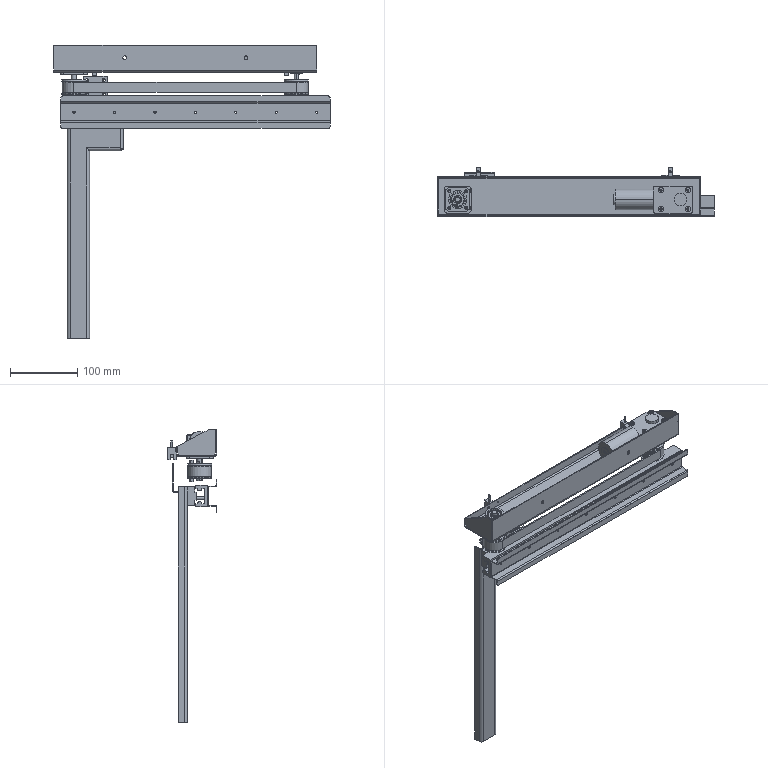Part | SolidWorks | 21 solids | 1204 faces | box 410 x 73.7 x 435 mm | volume 472209 mm3 | cylinder 763 | plane 392 | cone 29 | torus 16 | spline 4 | commonest cylinder face diameters 0.5 x88 6.55 x88 1.1 x80 8 x54 4.5 x50 27.33 x44